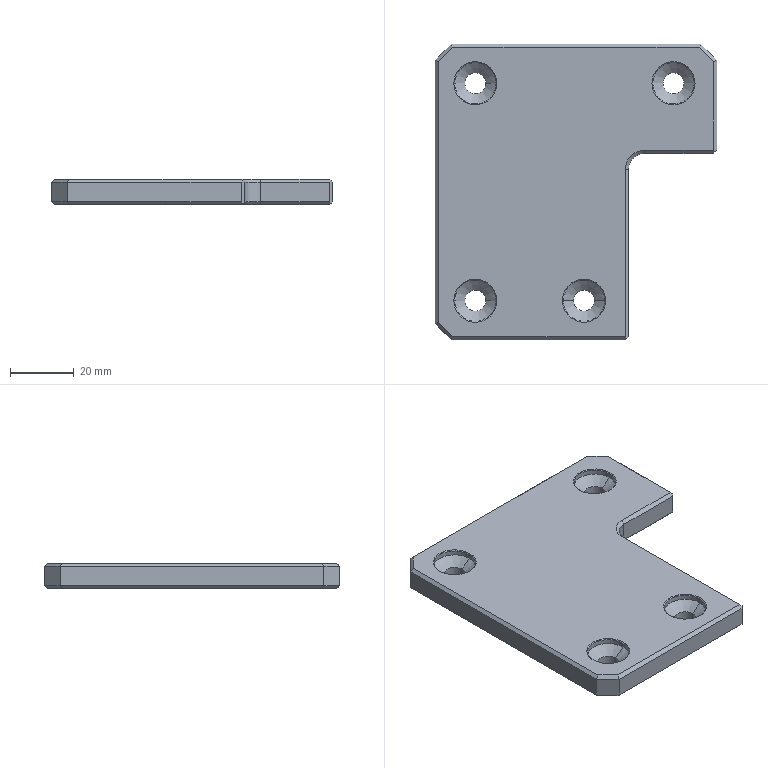Part | Creo | 1 solid | 68 faces | box 88 x 92.5 x 8 mm | volume 49408 mm3 | plane 33 | cone 18 | cylinder 17 | commonest cylinder face diameters 6.6 x8 13 x8 10 x1